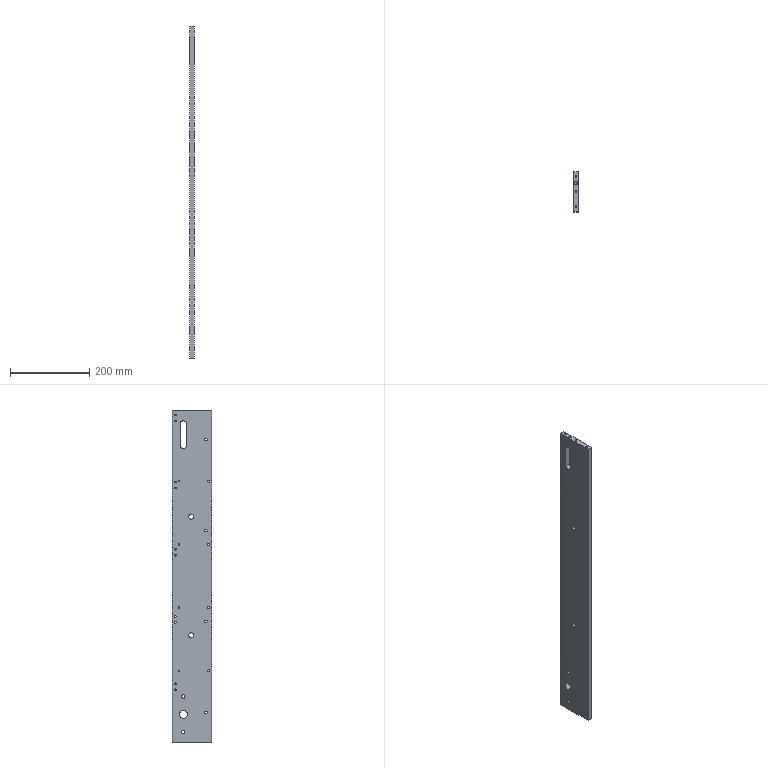Part | STEP file | 0228_201_Plate | 1 solid | 91 faces | box 12 x 100 x 840 mm | volume 978760 mm3 | cylinder 71 | cone 12 | plane 8 | commonest cylinder face diameters 4.2 x28 5 x20 6.8 x8 8.5 x4 12 x4 16 x3